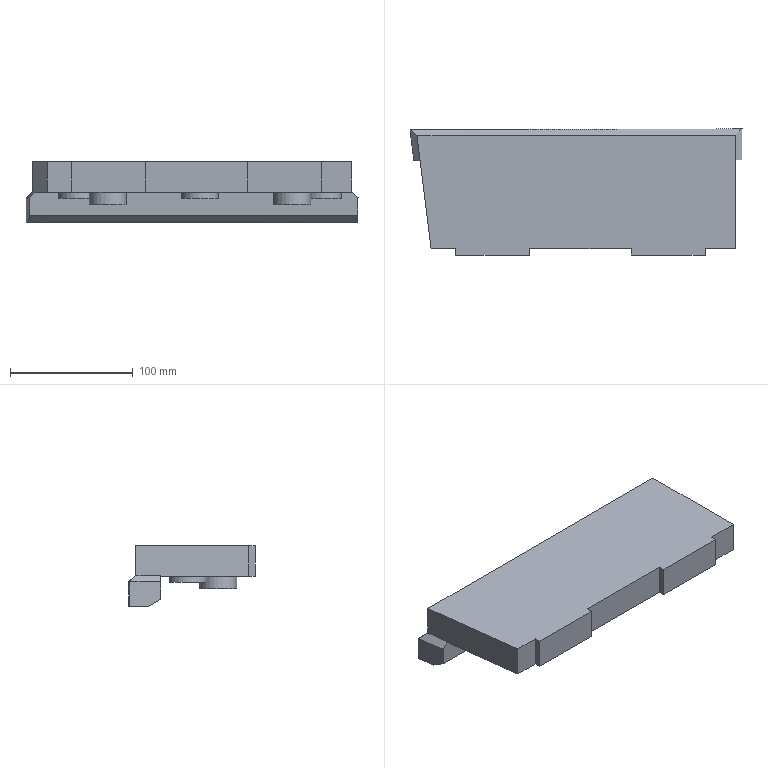Part | NX | features solid 2 | 1 solid | 33 faces | box 270.127 x 102.636 x 49.489 mm | volume 778285 mm3 | plane 22 | spline 6 | cylinder 5 | commonest cylinder face diameters 30 x5